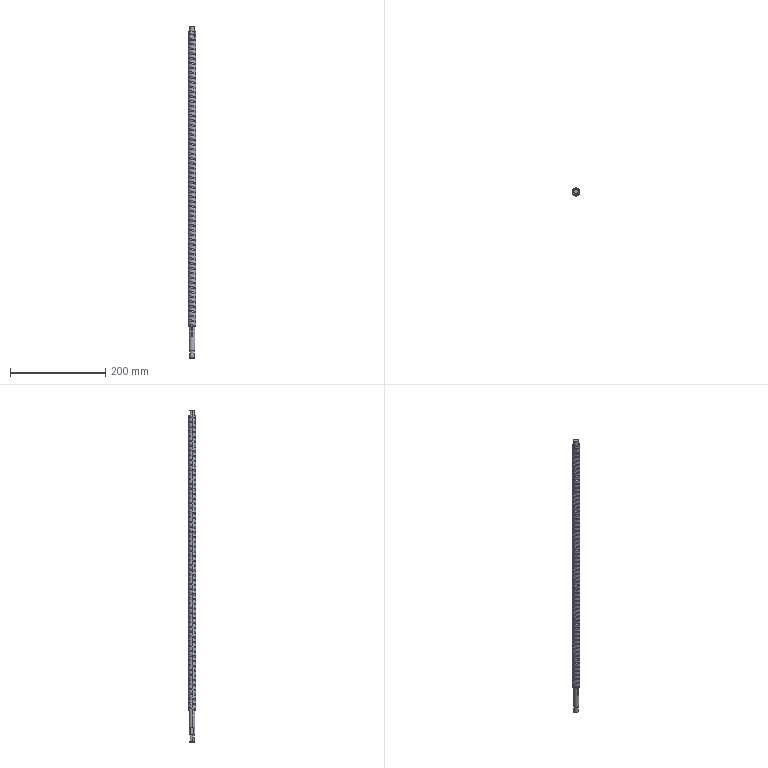Part | STEP file | Screw SFUL1605-696 | 1 solid | 164 faces | box 16 x 16 x 696 mm | volume 120509 mm3 | cylinder 137 | plane 20 | cone 6 | spline 1 | commonest cylinder face diameters 16 x128 10 x4 4 x3 12 x2